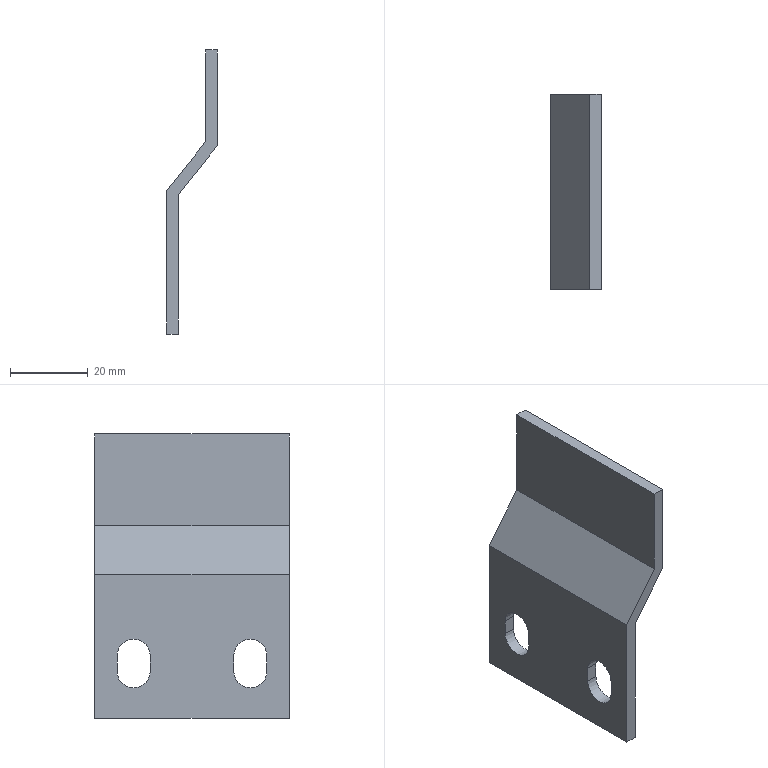Part | NX | features solid 2 | 1 solid | 18 faces | box 13 x 50 x 73 mm | volume 10929 mm3 | plane 14 | cylinder 4 | commonest cylinder face diameters 8.5 x4
STEP:
#1=CARTESIAN_POINT('',(-1145.,-370.,-15.));
#2=VERTEX_POINT('',#1);
#3=CARTESIAN_POINT('',(-1148.,-370.,-15.));
#4=VERTEX_POINT('',#3);
#5=CARTESIAN_POINT('',(-1145.,-370.,-15.));
#6=DIRECTION('',(-1.,0.,0.));
#7=VECTOR('',#6,1000.);
#8=LINE('',#5,#7);
#9=EDGE_CURVE('',#2,#4,#8,.T.);
#10=ORIENTED_EDGE('',*,*,#9,.T.);
#11=CARTESIAN_POINT('',(-1148.,-420.,-15.));
#12=VERTEX_POINT('',#11);
#13=CARTESIAN_POINT('',(-1148.,-445.,-15.));
#14=DIRECTION('',(0.,1.,0.));
#15=VECTOR('',#14,1000.);
#16=LINE('',#13,#15);
#17=EDGE_CURVE('',#12,#4,#16,.T.);
#18=ORIENTED_EDGE('',*,*,#17,.F.);
#19=CARTESIAN_POINT('',(-1145.,-420.,-15.));
#20=VERTEX_POINT('',#19);
#21=CARTESIAN_POINT('',(-1145.,-420.,-15.));
#22=DIRECTION('',(-1.,0.,0.));
#23=VECTOR('',#22,1000.);
#24=LINE('',#21,#23);
#25=EDGE_CURVE('',#20,#12,#24,.T.);
#26=ORIENTED_EDGE('',*,*,#25,.F.);
#27=CARTESIAN_POINT('',(-1145.,-445.,-15.));
#28=DIRECTION('',(0.,1.,0.));
#29=VECTOR('',#28,1000.);
#30=LINE('',#27,#29);
#31=EDGE_CURVE('',#20,#2,#30,.T.);
#32=ORIENTED_EDGE('',*,*,#31,.T.);
#33=EDGE_LOOP('',(#10,#18,#26,#32));
#34=FACE_BOUND('',#33,.T.);
#35=CARTESIAN_POINT('',(-1145.,-445.,-15.));
#36=DIRECTION('',(0.,0.,1.));
#37=DIRECTION('',(1.,0.,0.));
#38=AXIS2_PLACEMENT_3D('',#35,#36,#37);
#39=PLANE('',#38);
#40=ADVANCED_FACE('',(#34),#39,.T.);
#41=CARTESIAN_POINT('',(-1145.,-420.,-39.636));
#42=VERTEX_POINT('',#41);
#43=CARTESIAN_POINT('',(-1155.,-420.,-52.219));
#44=VERTEX_POINT('',#43);
#45=CARTESIAN_POINT('',(-1133.,-420.,-24.537));
#46=DIRECTION('',(-0.6222,0.,-0.7829));
#47=VECTOR('',#46,1000.);
#48=LINE('',#45,#47);
#49=EDGE_CURVE('',#42,#44,#48,.T.);
#50=ORIENTED_EDGE('',*,*,#49,.F.);
#51=CARTESIAN_POINT('',(-1145.,-420.,-15.));
#52=DIRECTION('',(0.,0.,-1.));
#53=VECTOR('',#52,1000.);
#54=LINE('',#51,#53);
#55=EDGE_CURVE('',#20,#42,#54,.T.);
#56=ORIENTED_EDGE('',*,*,#55,.F.);
#57=ORIENTED_EDGE('',*,*,#25,.T.);
#58=CARTESIAN_POINT('',(-1148.,-420.,-38.589));
#59=VERTEX_POINT('',#58);
#60=CARTESIAN_POINT('',(-1148.,-420.,-15.));
#61=DIRECTION('',(0.,0.,-1.));
#62=VECTOR('',#61,1000.);
#63=LINE('',#60,#62);
#64=EDGE_CURVE('',#12,#59,#63,.T.);
#65=ORIENTED_EDGE('',*,*,#64,.T.);
#66=CARTESIAN_POINT('',(-1158.,-420.,-51.172));
#67=VERTEX_POINT('',#66);
#68=CARTESIAN_POINT('',(-1159.174,-420.,-52.649));
#69=DIRECTION('',(0.6222,0.,0.7829));
#70=VECTOR('',#69,1000.);
#71=LINE('',#68,#70);
#72=EDGE_CURVE('',#67,#59,#71,.T.);
#73=ORIENTED_EDGE('',*,*,#72,.F.);
#74=CARTESIAN_POINT('',(-1158.,-420.,-88.));
#75=VERTEX_POINT('',#74);
#76=CARTESIAN_POINT('',(-1158.,-420.,-15.));
#77=DIRECTION('',(0.,0.,-1.));
#78=VECTOR('',#77,1000.);
#79=LINE('',#76,#78);
#80=EDGE_CURVE('',#67,#75,#79,.T.);
#81=ORIENTED_EDGE('',*,*,#80,.T.);
#82=CARTESIAN_POINT('',(-1155.,-420.,-88.));
#83=VERTEX_POINT('',#82);
#84=CARTESIAN_POINT('',(-1155.,-420.,-88.));
#85=DIRECTION('',(-1.,0.,0.));
#86=VECTOR('',#85,1000.);
#87=LINE('',#84,#86);
#88=EDGE_CURVE('',#83,#75,#87,.T.);
#89=ORIENTED_EDGE('',*,*,#88,.F.);
#90=CARTESIAN_POINT('',(-1155.,-420.,-55.));
#91=DIRECTION('',(0.,0.,-1.));
#92=VECTOR('',#91,1000.);
#93=LINE('',#90,#92);
#94=EDGE_CURVE('',#44,#83,#93,.T.);
#95=ORIENTED_EDGE('',*,*,#94,.F.);
#96=EDGE_LOOP('',(#50,#56,#57,#65,#73,#81,#89,#95));
#97=FACE_BOUND('',#96,.T.);
#98=CARTESIAN_POINT('',(-1145.,-420.,-15.));
#99=DIRECTION('',(0.,1.,0.));
#100=DIRECTION('',(0.,0.,-1.));
#101=AXIS2_PLACEMENT_3D('',#98,#99,#100);
#102=PLANE('',#101);
#103=ADVANCED_FACE('',(#97),#102,.F.);
#104=CARTESIAN_POINT('',(-1155.,-370.,-52.219));
#105=VERTEX_POINT('',#104);
#106=CARTESIAN_POINT('',(-1155.,-420.,-52.219));
#107=DIRECTION('',(0.,1.,0.));
#108=VECTOR('',#107,1000.);
#109=LINE('',#106,#108);
#110=EDGE_CURVE('',#44,#105,#109,.T.);
#111=ORIENTED_EDGE('',*,*,#110,.T.);
#112=CARTESIAN_POINT('',(-1145.,-370.,-39.636));
#113=VERTEX_POINT('',#112);
#114=CARTESIAN_POINT('',(-1156.826,-370.,-54.516));
#115=DIRECTION('',(-0.6222,0.,-0.7829));
#116=VECTOR('',#115,1000.);
#117=LINE('',#114,#116);
#118=EDGE_CURVE('',#113,#105,#117,.T.);
#119=ORIENTED_EDGE('',*,*,#118,.F.);
#120=CARTESIAN_POINT('',(-1145.,-420.,-39.636));
#121=DIRECTION('',(0.,1.,0.));
#122=VECTOR('',#121,1000.);
#123=LINE('',#120,#122);
#124=EDGE_CURVE('',#42,#113,#123,.T.);
#125=ORIENTED_EDGE('',*,*,#124,.F.);
#126=ORIENTED_EDGE('',*,*,#49,.T.);
#127=EDGE_LOOP('',(#111,#119,#125,#126));
#128=FACE_BOUND('',#127,.T.);
#129=CARTESIAN_POINT('',(-1156.826,-420.,-54.516));
#130=DIRECTION('',(0.7829,0.,-0.6222));
#131=DIRECTION('',(-0.6222,0.,-0.7829));
#132=AXIS2_PLACEMENT_3D('',#129,#130,#131);
#133=PLANE('',#132);
#134=ADVANCED_FACE('',(#128),#133,.T.);
#135=CARTESIAN_POINT('',(-1148.,-370.,-38.589));
#136=VERTEX_POINT('',#135);
#137=CARTESIAN_POINT('',(-1148.,-370.,-15.));
#138=DIRECTION('',(0.,0.,-1.));
#139=VECTOR('',#138,1000.);
#140=LINE('',#137,#139);
#141=EDGE_CURVE('',#4,#136,#140,.T.);
#142=ORIENTED_EDGE('',*,*,#141,.F.);
#143=ORIENTED_EDGE('',*,*,#9,.F.);
#144=CARTESIAN_POINT('',(-1145.,-370.,-15.));
#145=DIRECTION('',(0.,0.,-1.));
#146=VECTOR('',#145,1000.);
#147=LINE('',#144,#146);
#148=EDGE_CURVE('',#2,#113,#147,.T.);
#149=ORIENTED_EDGE('',*,*,#148,.T.);
#150=ORIENTED_EDGE('',*,*,#118,.T.);
#151=CARTESIAN_POINT('',(-1155.,-370.,-88.));
#152=VERTEX_POINT('',#151);
#153=CARTESIAN_POINT('',(-1155.,-370.,-55.));
#154=DIRECTION('',(0.,0.,-1.));
#155=VECTOR('',#154,1000.);
#156=LINE('',#153,#155);
#157=EDGE_CURVE('',#105,#152,#156,.T.);
#158=ORIENTED_EDGE('',*,*,#157,.T.);
#159=CARTESIAN_POINT('',(-1158.,-370.,-88.));
#160=VERTEX_POINT('',#159);
#161=CARTESIAN_POINT('',(-1155.,-370.,-88.));
#162=DIRECTION('',(-1.,0.,0.));
#163=VECTOR('',#162,1000.);
#164=LINE('',#161,#163);
#165=EDGE_CURVE('',#152,#160,#164,.T.);
#166=ORIENTED_EDGE('',*,*,#165,.T.);
#167=CARTESIAN_POINT('',(-1158.,-370.,-51.172));
#168=VERTEX_POINT('',#167);
#169=CARTESIAN_POINT('',(-1158.,-370.,-55.));
#170=DIRECTION('',(0.,0.,-1.));
#171=VECTOR('',#170,1000.);
#172=LINE('',#169,#171);
#173=EDGE_CURVE('',#168,#160,#172,.T.);
#174=ORIENTED_EDGE('',*,*,#173,.F.);
#175=CARTESIAN_POINT('',(-1135.349,-370.,-22.67));
#176=DIRECTION('',(0.6222,0.,0.7829));
#177=VECTOR('',#176,1000.);
#178=LINE('',#175,#177);
#179=EDGE_CURVE('',#168,#136,#178,.T.);
#180=ORIENTED_EDGE('',*,*,#179,.T.);
#181=EDGE_LOOP('',(#142,#143,#149,#150,#158,#166,#174,#180));
#182=FACE_BOUND('',#181,.T.);
#183=CARTESIAN_POINT('',(-1145.,-370.,-15.));
#184=DIRECTION('',(0.,1.,0.));
#185=DIRECTION('',(0.,0.,-1.));
#186=AXIS2_PLACEMENT_3D('',#183,#184,#185);
#187=PLANE('',#186);
#188=ADVANCED_FACE('',(#182),#187,.T.);
#189=ORIENTED_EDGE('',*,*,#64,.F.);
#190=ORIENTED_EDGE('',*,*,#17,.T.);
#191=ORIENTED_EDGE('',*,*,#141,.T.);
#192=CARTESIAN_POINT('',(-1148.,-420.,-38.589));
#193=DIRECTION('',(0.,1.,0.));
#194=VECTOR('',#193,1000.);
#195=LINE('',#192,#194);
#196=EDGE_CURVE('',#59,#136,#195,.T.);
#197=ORIENTED_EDGE('',*,*,#196,.F.);
#198=EDGE_LOOP('',(#189,#190,#191,#197));
#199=FACE_BOUND('',#198,.T.);
#200=CARTESIAN_POINT('',(-1148.,-445.,-15.));
#201=DIRECTION('',(1.,0.,0.));
#202=DIRECTION('',(0.,0.,-1.));
#203=AXIS2_PLACEMENT_3D('',#200,#201,#202);
#204=PLANE('',#203);
#205=ADVANCED_FACE('',(#199),#204,.F.);
#206=ORIENTED_EDGE('',*,*,#124,.T.);
#207=ORIENTED_EDGE('',*,*,#148,.F.);
#208=ORIENTED_EDGE('',*,*,#31,.F.);
#209=ORIENTED_EDGE('',*,*,#55,.T.);
#210=EDGE_LOOP('',(#206,#207,#208,#209));
#211=FACE_BOUND('',#210,.T.);
#212=CARTESIAN_POINT('',(-1145.,-445.,-15.));
#213=DIRECTION('',(1.,0.,0.));
#214=DIRECTION('',(0.,0.,-1.));
#215=AXIS2_PLACEMENT_3D('',#212,#213,#214);
#216=PLANE('',#215);
#217=ADVANCED_FACE('',(#211),#216,.T.);
#218=ORIENTED_EDGE('',*,*,#196,.T.);
#219=ORIENTED_EDGE('',*,*,#179,.F.);
#220=CARTESIAN_POINT('',(-1158.,-420.,-51.172));
#221=DIRECTION('',(0.,1.,0.));
#222=VECTOR('',#221,1000.);
#223=LINE('',#220,#222);
#224=EDGE_CURVE('',#67,#168,#223,.T.);
#225=ORIENTED_EDGE('',*,*,#224,.F.);
#226=ORIENTED_EDGE('',*,*,#72,.T.);
#227=EDGE_LOOP('',(#218,#219,#225,#226));
#228=FACE_BOUND('',#227,.T.);
#229=CARTESIAN_POINT('',(-1159.174,-420.,-52.649));
#230=DIRECTION('',(0.7829,0.,-0.6222));
#231=DIRECTION('',(-0.6222,0.,-0.7829));
#232=AXIS2_PLACEMENT_3D('',#229,#230,#231);
#233=PLANE('',#232);
#234=ADVANCED_FACE('',(#228),#233,.F.);
#235=CARTESIAN_POINT('',(-1158.,-405.75,-76.));
#236=VERTEX_POINT('',#235);
#237=CARTESIAN_POINT('',(-1158.,-405.75,-72.));
#238=VERTEX_POINT('',#237);
#239=CARTESIAN_POINT('',(-1158.,-405.75,-80.25));
#240=DIRECTION('',(0.,0.,1.));
#241=VECTOR('',#240,1000.);
#242=LINE('',#239,#241);
#243=EDGE_CURVE('',#236,#238,#242,.T.);
#244=ORIENTED_EDGE('',*,*,#243,.T.);
#245=CARTESIAN_POINT('',(-1158.,-414.25,-72.));
#246=VERTEX_POINT('',#245);
#247=CARTESIAN_POINT('',(-1158.,-410.,-72.));
#248=DIRECTION('',(1.,0.,0.));
#249=DIRECTION('',(0.,0.,1.));
#250=AXIS2_PLACEMENT_3D('',#247,#248,#249);
#251=CIRCLE('',#250,4.25);
#252=EDGE_CURVE('',#238,#246,#251,.T.);
#253=ORIENTED_EDGE('',*,*,#252,.T.);
#254=CARTESIAN_POINT('',(-1158.,-414.25,-76.));
#255=VERTEX_POINT('',#254);
#256=CARTESIAN_POINT('',(-1158.,-414.25,-80.25));
#257=DIRECTION('',(0.,0.,1.));
#258=VECTOR('',#257,1000.);
#259=LINE('',#256,#258);
#260=EDGE_CURVE('',#255,#246,#259,.T.);
#261=ORIENTED_EDGE('',*,*,#260,.F.);
#262=CARTESIAN_POINT('',(-1158.,-410.,-76.));
#263=DIRECTION('',(1.,0.,0.));
#264=DIRECTION('',(0.,0.,1.));
#265=AXIS2_PLACEMENT_3D('',#262,#263,#264);
#266=CIRCLE('',#265,4.25);
#267=EDGE_CURVE('',#255,#236,#266,.T.);
#268=ORIENTED_EDGE('',*,*,#267,.T.);
#269=EDGE_LOOP('',(#244,#253,#261,#268));
#270=FACE_BOUND('',#269,.T.);
#271=CARTESIAN_POINT('',(-1158.,-375.75,-76.));
#272=VERTEX_POINT('',#271);
#273=CARTESIAN_POINT('',(-1158.,-375.75,-72.));
#274=VERTEX_POINT('',#273);
#275=CARTESIAN_POINT('',(-1158.,-375.75,-80.25));
#276=DIRECTION('',(0.,0.,1.));
#277=VECTOR('',#276,1000.);
#278=LINE('',#275,#277);
#279=EDGE_CURVE('',#272,#274,#278,.T.);
#280=ORIENTED_EDGE('',*,*,#279,.T.);
#281=CARTESIAN_POINT('',(-1158.,-384.25,-72.));
#282=VERTEX_POINT('',#281);
#283=CARTESIAN_POINT('',(-1158.,-380.,-72.));
#284=DIRECTION('',(1.,0.,0.));
#285=DIRECTION('',(0.,0.,1.));
#286=AXIS2_PLACEMENT_3D('',#283,#284,#285);
#287=CIRCLE('',#286,4.25);
#288=EDGE_CURVE('',#274,#282,#287,.T.);
#289=ORIENTED_EDGE('',*,*,#288,.T.);
#290=CARTESIAN_POINT('',(-1158.,-384.25,-76.));
#291=VERTEX_POINT('',#290);
#292=CARTESIAN_POINT('',(-1158.,-384.25,-80.25));
#293=DIRECTION('',(0.,0.,1.));
#294=VECTOR('',#293,1000.);
#295=LINE('',#292,#294);
#296=EDGE_CURVE('',#291,#282,#295,.T.);
#297=ORIENTED_EDGE('',*,*,#296,.F.);
#298=CARTESIAN_POINT('',(-1158.,-380.,-76.));
#299=DIRECTION('',(1.,0.,0.));
#300=DIRECTION('',(0.,0.,1.));
#301=AXIS2_PLACEMENT_3D('',#298,#299,#300);
#302=CIRCLE('',#301,4.25);
#303=EDGE_CURVE('',#291,#272,#302,.T.);
#304=ORIENTED_EDGE('',*,*,#303,.T.);
#305=EDGE_LOOP('',(#280,#289,#297,#304));
#306=FACE_BOUND('',#305,.T.);
#307=ORIENTED_EDGE('',*,*,#80,.F.);
#308=ORIENTED_EDGE('',*,*,#224,.T.);
#309=ORIENTED_EDGE('',*,*,#173,.T.);
#310=CARTESIAN_POINT('',(-1158.,-445.,-88.));
#311=DIRECTION('',(0.,1.,0.));
#312=VECTOR('',#311,1000.);
#313=LINE('',#310,#312);
#314=EDGE_CURVE('',#75,#160,#313,.T.);
#315=ORIENTED_EDGE('',*,*,#314,.F.);
#316=EDGE_LOOP('',(#307,#308,#309,#315));
#317=FACE_BOUND('',#316,.T.);
#318=CARTESIAN_POINT('',(-1158.,-445.,-55.));
#319=DIRECTION('',(1.,0.,0.));
#320=DIRECTION('',(0.,0.,-1.));
#321=AXIS2_PLACEMENT_3D('',#318,#319,#320);
#322=PLANE('',#321);
#323=ADVANCED_FACE('',(#270,#306,#317),#322,.F.);
#324=ORIENTED_EDGE('',*,*,#88,.T.);
#325=ORIENTED_EDGE('',*,*,#314,.T.);
#326=ORIENTED_EDGE('',*,*,#165,.F.);
#327=CARTESIAN_POINT('',(-1155.,-445.,-88.));
#328=DIRECTION('',(0.,1.,0.));
#329=VECTOR('',#328,1000.);
#330=LINE('',#327,#329);
#331=EDGE_CURVE('',#83,#152,#330,.T.);
#332=ORIENTED_EDGE('',*,*,#331,.F.);
#333=EDGE_LOOP('',(#324,#325,#326,#332));
#334=FACE_BOUND('',#333,.T.);
#335=CARTESIAN_POINT('',(-1155.,-445.,-88.));
#336=DIRECTION('',(0.,0.,1.));
#337=DIRECTION('',(1.,0.,0.));
#338=AXIS2_PLACEMENT_3D('',#335,#336,#337);
#339=PLANE('',#338);
#340=ADVANCED_FACE('',(#334),#339,.F.);
#341=CARTESIAN_POINT('',(-1155.,-405.75,-76.));
#342=VERTEX_POINT('',#341);
#343=CARTESIAN_POINT('',(-1155.,-414.25,-76.));
#344=VERTEX_POINT('',#343);
#345=CARTESIAN_POINT('',(-1155.,-410.,-76.));
#346=DIRECTION('',(-1.,0.,0.));
#347=DIRECTION('',(0.,0.,-1.));
#348=AXIS2_PLACEMENT_3D('',#345,#346,#347);
#349=CIRCLE('',#348,4.25);
#350=EDGE_CURVE('',#342,#344,#349,.T.);
#351=ORIENTED_EDGE('',*,*,#350,.T.);
#352=CARTESIAN_POINT('',(-1155.,-414.25,-72.));
#353=VERTEX_POINT('',#352);
#354=CARTESIAN_POINT('',(-1155.,-414.25,-57.75));
#355=DIRECTION('',(0.,0.,-1.));
#356=VECTOR('',#355,1000.);
#357=LINE('',#354,#356);
#358=EDGE_CURVE('',#353,#344,#357,.T.);
#359=ORIENTED_EDGE('',*,*,#358,.F.);
#360=CARTESIAN_POINT('',(-1155.,-405.75,-72.));
#361=VERTEX_POINT('',#360);
#362=CARTESIAN_POINT('',(-1155.,-410.,-72.));
#363=DIRECTION('',(-1.,0.,0.));
#364=DIRECTION('',(0.,0.,-1.));
#365=AXIS2_PLACEMENT_3D('',#362,#363,#364);
#366=CIRCLE('',#365,4.25);
#367=EDGE_CURVE('',#353,#361,#366,.T.);
#368=ORIENTED_EDGE('',*,*,#367,.T.);
#369=CARTESIAN_POINT('',(-1155.,-405.75,-57.75));
#370=DIRECTION('',(0.,0.,1.));
#371=VECTOR('',#370,1000.);
#372=LINE('',#369,#371);
#373=EDGE_CURVE('',#342,#361,#372,.T.);
#374=ORIENTED_EDGE('',*,*,#373,.F.);
#375=EDGE_LOOP('',(#351,#359,#368,#374));
#376=FACE_BOUND('',#375,.T.);
#377=CARTESIAN_POINT('',(-1155.,-375.75,-76.));
#378=VERTEX_POINT('',#377);
#379=CARTESIAN_POINT('',(-1155.,-384.25,-76.));
#380=VERTEX_POINT('',#379);
#381=CARTESIAN_POINT('',(-1155.,-380.,-76.));
#382=DIRECTION('',(-1.,0.,0.));
#383=DIRECTION('',(0.,0.,-1.));
#384=AXIS2_PLACEMENT_3D('',#381,#382,#383);
#385=CIRCLE('',#384,4.25);
#386=EDGE_CURVE('',#378,#380,#385,.T.);
#387=ORIENTED_EDGE('',*,*,#386,.T.);
#388=CARTESIAN_POINT('',(-1155.,-384.25,-72.));
#389=VERTEX_POINT('',#388);
#390=CARTESIAN_POINT('',(-1155.,-384.25,-57.75));
#391=DIRECTION('',(0.,0.,-1.));
#392=VECTOR('',#391,1000.);
#393=LINE('',#390,#392);
#394=EDGE_CURVE('',#389,#380,#393,.T.);
#395=ORIENTED_EDGE('',*,*,#394,.F.);
#396=CARTESIAN_POINT('',(-1155.,-375.75,-72.));
#397=VERTEX_POINT('',#396);
#398=CARTESIAN_POINT('',(-1155.,-380.,-72.));
#399=DIRECTION('',(-1.,0.,0.));
#400=DIRECTION('',(0.,0.,-1.));
#401=AXIS2_PLACEMENT_3D('',#398,#399,#400);
#402=CIRCLE('',#401,4.25);
#403=EDGE_CURVE('',#389,#397,#402,.T.);
#404=ORIENTED_EDGE('',*,*,#403,.T.);
#405=CARTESIAN_POINT('',(-1155.,-375.75,-57.75));
#406=DIRECTION('',(0.,0.,1.));
#407=VECTOR('',#406,1000.);
#408=LINE('',#405,#407);
#409=EDGE_CURVE('',#378,#397,#408,.T.);
#410=ORIENTED_EDGE('',*,*,#409,.F.);
#411=EDGE_LOOP('',(#387,#395,#404,#410));
#412=FACE_BOUND('',#411,.T.);
#413=ORIENTED_EDGE('',*,*,#94,.T.);
#414=ORIENTED_EDGE('',*,*,#331,.T.);
#415=ORIENTED_EDGE('',*,*,#157,.F.);
#416=ORIENTED_EDGE('',*,*,#110,.F.);
#417=EDGE_LOOP('',(#413,#414,#415,#416));
#418=FACE_BOUND('',#417,.T.);
#419=CARTESIAN_POINT('',(-1155.,-445.,-55.));
#420=DIRECTION('',(1.,0.,0.));
#421=DIRECTION('',(0.,0.,-1.));
#422=AXIS2_PLACEMENT_3D('',#419,#420,#421);
#423=PLANE('',#422);
#424=ADVANCED_FACE('',(#376,#412,#418),#423,.T.);
#425=CARTESIAN_POINT('',(-1158.,-375.75,-76.));
#426=DIRECTION('',(1.,0.,0.));
#427=VECTOR('',#426,1000.);
#428=LINE('',#425,#427);
#429=EDGE_CURVE('',#272,#378,#428,.T.);
#430=ORIENTED_EDGE('',*,*,#429,.T.);
#431=ORIENTED_EDGE('',*,*,#409,.T.);
#432=CARTESIAN_POINT('',(-1158.,-375.75,-72.));
#433=DIRECTION('',(-1.,0.,0.));
#434=VECTOR('',#433,1000.);
#435=LINE('',#432,#434);
#436=EDGE_CURVE('',#397,#274,#435,.T.);
#437=ORIENTED_EDGE('',*,*,#436,.T.);
#438=ORIENTED_EDGE('',*,*,#279,.F.);
#439=EDGE_LOOP('',(#430,#431,#437,#438));
#440=FACE_BOUND('',#439,.T.);
#441=CARTESIAN_POINT('',(-1158.,-375.75,-80.25));
#442=DIRECTION('',(0.,1.,0.));
#443=DIRECTION('',(0.,0.,-1.));
#444=AXIS2_PLACEMENT_3D('',#441,#442,#443);
#445=PLANE('',#444);
#446=ADVANCED_FACE('',(#440),#445,.F.);
#447=CARTESIAN_POINT('',(-1158.,-384.25,-72.));
#448=DIRECTION('',(1.,0.,0.));
#449=VECTOR('',#448,1000.);
#450=LINE('',#447,#449);
#451=EDGE_CURVE('',#282,#389,#450,.T.);
#452=ORIENTED_EDGE('',*,*,#451,.T.);
#453=ORIENTED_EDGE('',*,*,#394,.T.);
#454=CARTESIAN_POINT('',(-1158.,-384.25,-76.));
#455=DIRECTION('',(-1.,0.,0.));
#456=VECTOR('',#455,1000.);
#457=LINE('',#454,#456);
#458=EDGE_CURVE('',#380,#291,#457,.T.);
#459=ORIENTED_EDGE('',*,*,#458,.T.);
#460=ORIENTED_EDGE('',*,*,#296,.T.);
#461=EDGE_LOOP('',(#452,#453,#459,#460));
#462=FACE_BOUND('',#461,.T.);
#463=CARTESIAN_POINT('',(-1158.,-384.25,-80.25));
#464=DIRECTION('',(0.,1.,0.));
#465=DIRECTION('',(0.,0.,-1.));
#466=AXIS2_PLACEMENT_3D('',#463,#464,#465);
#467=PLANE('',#466);
#468=ADVANCED_FACE('',(#462),#467,.T.);
#469=ORIENTED_EDGE('',*,*,#386,.F.);
#470=ORIENTED_EDGE('',*,*,#429,.F.);
#471=ORIENTED_EDGE('',*,*,#303,.F.);
#472=ORIENTED_EDGE('',*,*,#458,.F.);
#473=EDGE_LOOP('',(#469,#470,#471,#472));
#474=FACE_BOUND('',#473,.T.);
#475=CARTESIAN_POINT('',(-1158.,-380.,-76.));
#476=DIRECTION('',(1.,0.,0.));
#477=DIRECTION('',(0.,0.,-1.));
#478=AXIS2_PLACEMENT_3D('',#475,#476,#477);
#479=CYLINDRICAL_SURFACE('',#478,4.25);
#480=ADVANCED_FACE('',(#474),#479,.F.);
#481=ORIENTED_EDGE('',*,*,#403,.F.);
#482=ORIENTED_EDGE('',*,*,#451,.F.);
#483=ORIENTED_EDGE('',*,*,#288,.F.);
#484=ORIENTED_EDGE('',*,*,#436,.F.);
#485=EDGE_LOOP('',(#481,#482,#483,#484));
#486=FACE_BOUND('',#485,.T.);
#487=CARTESIAN_POINT('',(-1158.,-380.,-72.));
#488=DIRECTION('',(-1.,0.,0.));
#489=DIRECTION('',(0.,0.,1.));
#490=AXIS2_PLACEMENT_3D('',#487,#488,#489);
#491=CYLINDRICAL_SURFACE('',#490,4.25);
#492=ADVANCED_FACE('',(#486),#491,.F.);
#493=CARTESIAN_POINT('',(-1158.,-414.25,-72.));
#494=DIRECTION('',(1.,0.,0.));
#495=VECTOR('',#494,1000.);
#496=LINE('',#493,#495);
#497=EDGE_CURVE('',#246,#353,#496,.T.);
#498=ORIENTED_EDGE('',*,*,#497,.T.);
#499=ORIENTED_EDGE('',*,*,#358,.T.);
#500=CARTESIAN_POINT('',(-1158.,-414.25,-76.));
#501=DIRECTION('',(-1.,0.,0.));
#502=VECTOR('',#501,1000.);
#503=LINE('',#500,#502);
#504=EDGE_CURVE('',#344,#255,#503,.T.);
#505=ORIENTED_EDGE('',*,*,#504,.T.);
#506=ORIENTED_EDGE('',*,*,#260,.T.);
#507=EDGE_LOOP('',(#498,#499,#505,#506));
#508=FACE_BOUND('',#507,.T.);
#509=CARTESIAN_POINT('',(-1158.,-414.25,-80.25));
#510=DIRECTION('',(0.,-1.,0.));
#511=DIRECTION('',(0.,0.,1.));
#512=AXIS2_PLACEMENT_3D('',#509,#510,#511);
#513=PLANE('',#512);
#514=ADVANCED_FACE('',(#508),#513,.F.);
#515=CARTESIAN_POINT('',(-1158.,-405.75,-76.));
#516=DIRECTION('',(1.,0.,0.));
#517=VECTOR('',#516,1000.);
#518=LINE('',#515,#517);
#519=EDGE_CURVE('',#236,#342,#518,.T.);
#520=ORIENTED_EDGE('',*,*,#519,.T.);
#521=ORIENTED_EDGE('',*,*,#373,.T.);
#522=CARTESIAN_POINT('',(-1158.,-405.75,-72.));
#523=DIRECTION('',(-1.,0.,0.));
#524=VECTOR('',#523,1000.);
#525=LINE('',#522,#524);
#526=EDGE_CURVE('',#361,#238,#525,.T.);
#527=ORIENTED_EDGE('',*,*,#526,.T.);
#528=ORIENTED_EDGE('',*,*,#243,.F.);
#529=EDGE_LOOP('',(#520,#521,#527,#528));
#530=FACE_BOUND('',#529,.T.);
#531=CARTESIAN_POINT('',(-1158.,-405.75,-80.25));
#532=DIRECTION('',(0.,-1.,0.));
#533=DIRECTION('',(0.,0.,1.));
#534=AXIS2_PLACEMENT_3D('',#531,#532,#533);
#535=PLANE('',#534);
#536=ADVANCED_FACE('',(#530),#535,.T.);
#537=ORIENTED_EDGE('',*,*,#350,.F.);
#538=ORIENTED_EDGE('',*,*,#519,.F.);
#539=ORIENTED_EDGE('',*,*,#267,.F.);
#540=ORIENTED_EDGE('',*,*,#504,.F.);
#541=EDGE_LOOP('',(#537,#538,#539,#540));
#542=FACE_BOUND('',#541,.T.);
#543=CARTESIAN_POINT('',(-1158.,-410.,-76.));
#544=DIRECTION('',(-1.,0.,0.));
#545=DIRECTION('',(0.,0.,1.));
#546=AXIS2_PLACEMENT_3D('',#543,#544,#545);
#547=CYLINDRICAL_SURFACE('',#546,4.25);
#548=ADVANCED_FACE('',(#542),#547,.F.);
#549=ORIENTED_EDGE('',*,*,#367,.F.);
#550=ORIENTED_EDGE('',*,*,#497,.F.);
#551=ORIENTED_EDGE('',*,*,#252,.F.);
#552=ORIENTED_EDGE('',*,*,#526,.F.);
#553=EDGE_LOOP('',(#549,#550,#551,#552));
#554=FACE_BOUND('',#553,.T.);
#555=CARTESIAN_POINT('',(-1158.,-410.,-72.));
#556=DIRECTION('',(1.,0.,0.));
#557=DIRECTION('',(0.,0.,-1.));
#558=AXIS2_PLACEMENT_3D('',#555,#556,#557);
#559=CYLINDRICAL_SURFACE('',#558,4.25);
#560=ADVANCED_FACE('',(#554),#559,.F.);
#561=CLOSED_SHELL('',(#40,#103,#134,#188,#205,#217,#234,#323,#340,#424,#446,#468,#480,#492,#514,#536,#548,#560));
#562=MANIFOLD_SOLID_BREP('',#561);
#563=(LENGTH_UNIT()NAMED_UNIT(*)SI_UNIT(.MILLI.,.METRE.));
#564=UNCERTAINTY_MEASURE_WITH_UNIT(LENGTH_MEASURE(0.00001),#563,'','');
#565=(NAMED_UNIT(*)PLANE_ANGLE_UNIT()SI_UNIT($,.RADIAN.));
#566=(NAMED_UNIT(*)SI_UNIT($,.STERADIAN.)SOLID_ANGLE_UNIT());
#567=(GEOMETRIC_REPRESENTATION_CONTEXT(3)GLOBAL_UNCERTAINTY_ASSIGNED_CONTEXT((#564))GLOBAL_UNIT_ASSIGNED_CONTEXT((#563,#565,#566))REPRESENTATION_CONTEXT('',''));
#568=ADVANCED_BREP_SHAPE_REPRESENTATION('',(#562),#567);